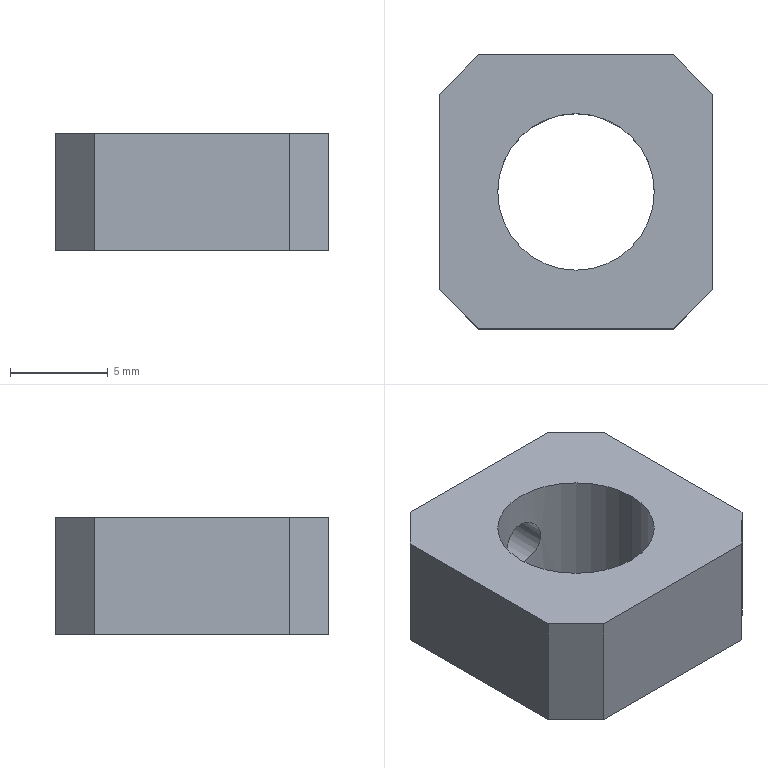Part | SolidWorks | features 3DProfileFeature 1, Chamfer 1, Extrusion 1, HoleWzd 1 | 1 solid | 14 faces | box 14 x 14 x 6 mm | volume 811.438 mm3 | plane 10 | cylinder 4 | commonest cylinder face diameters 2.5 x2 8 x2
STEP:
#1=CARTESIAN_POINT('',(0.,4.,1.25));
#2=VERTEX_POINT('',#1);
#3=CARTESIAN_POINT('',(0.,4.,-1.25));
#4=VERTEX_POINT('',#3);
#5=CARTESIAN_POINT('',(0.,4.,1.25));
#6=CARTESIAN_POINT('',(-0.1663,4.,1.25));
#7=CARTESIAN_POINT('',(-0.3294,3.989,1.217));
#8=CARTESIAN_POINT('',(-0.6318,3.953,1.091));
#9=CARTESIAN_POINT('',(-0.7697,3.927,0.9981));
#10=CARTESIAN_POINT('',(-0.9987,3.875,0.7689));
#11=CARTESIAN_POINT('',(-1.092,3.849,0.6304));
#12=CARTESIAN_POINT('',(-1.217,3.811,0.33));
#13=CARTESIAN_POINT('',(-1.25,3.8,0.1648));
#14=CARTESIAN_POINT('',(-1.25,3.8,-0.08153));
#15=CARTESIAN_POINT('',(-1.242,3.802,-0.165));
#16=CARTESIAN_POINT('',(-1.21,3.813,-0.3257));
#17=CARTESIAN_POINT('',(-1.186,3.82,-0.4039));
#18=CARTESIAN_POINT('',(-1.091,3.849,-0.6319));
#19=CARTESIAN_POINT('',(-0.9989,3.875,-0.769));
#20=CARTESIAN_POINT('',(-0.8259,3.914,-0.9418));
#21=CARTESIAN_POINT('',(-0.7634,3.927,-0.9932));
#22=CARTESIAN_POINT('',(-0.6283,3.951,-1.084));
#23=CARTESIAN_POINT('',(-0.5551,3.962,-1.123));
#24=CARTESIAN_POINT('',(-0.3291,3.989,-1.217));
#25=CARTESIAN_POINT('',(-0.1639,4.,-1.25));
#26=CARTESIAN_POINT('',(0.,4.,-1.25));
#27=B_SPLINE_CURVE_WITH_KNOTS('',3,(#5,#6,#7,#8,#9,#10,#11,#12,#13,#14,#15,#16,#17,#18,#19,#20,#21,#22,#23,#24,#25,#26),.UNSPECIFIED.,.F.,.F.,(4,2,2,2,2,2,2,2,2,2,4),(0.,0.0004916,0.0009832,0.001475,0.001966,0.002212,0.002458,0.00295,0.003195,0.003441,0.003933),.UNSPECIFIED.);
#28=EDGE_CURVE('',#2,#4,#27,.T.);
#29=ORIENTED_EDGE('',*,*,#28,.T.);
#30=CARTESIAN_POINT('',(0.,7.,-1.25));
#31=VERTEX_POINT('',#30);
#32=CARTESIAN_POINT('',(0.,7.,-1.25));
#33=DIRECTION('',(0.,1.,0.));
#34=VECTOR('',#33,1000.);
#35=LINE('',#32,#34);
#36=EDGE_CURVE('',#4,#31,#35,.T.);
#37=ORIENTED_EDGE('',*,*,#36,.T.);
#38=CARTESIAN_POINT('',(0.,7.,1.25));
#39=VERTEX_POINT('',#38);
#40=CARTESIAN_POINT('',(0.,7.,0.));
#41=DIRECTION('',(0.,1.,0.));
#42=DIRECTION('',(0.,0.,1.));
#43=AXIS2_PLACEMENT_3D('',#40,#41,#42);
#44=CIRCLE('',#43,1.25);
#45=EDGE_CURVE('',#31,#39,#44,.T.);
#46=ORIENTED_EDGE('',*,*,#45,.T.);
#47=CARTESIAN_POINT('',(0.,7.,1.25));
#48=DIRECTION('',(0.,1.,0.));
#49=VECTOR('',#48,1000.);
#50=LINE('',#47,#49);
#51=EDGE_CURVE('',#2,#39,#50,.T.);
#52=ORIENTED_EDGE('',*,*,#51,.F.);
#53=EDGE_LOOP('',(#29,#37,#46,#52));
#54=FACE_OUTER_BOUND('',#53,.T.);
#55=CARTESIAN_POINT('',(0.,7.,0.));
#56=DIRECTION('',(0.,1.,0.));
#57=DIRECTION('',(0.,0.,1.));
#58=AXIS2_PLACEMENT_3D('',#55,#56,#57);
#59=CYLINDRICAL_SURFACE('',#58,1.25);
#60=ADVANCED_FACE('',(#54),#59,.F.);
#61=CARTESIAN_POINT('',(-4.,0.,3.));
#62=VERTEX_POINT('',#61);
#63=CARTESIAN_POINT('',(4.,0.,3.));
#64=VERTEX_POINT('',#63);
#65=CARTESIAN_POINT('',(0.,0.,3.));
#66=DIRECTION('',(0.,0.,1.));
#67=DIRECTION('',(1.,0.,0.));
#68=AXIS2_PLACEMENT_3D('',#65,#66,#67);
#69=CIRCLE('',#68,4.);
#70=EDGE_CURVE('',#62,#64,#69,.T.);
#71=ORIENTED_EDGE('',*,*,#70,.T.);
#72=CARTESIAN_POINT('',(4.,0.,-3.));
#73=VERTEX_POINT('',#72);
#74=CARTESIAN_POINT('',(4.,0.,3.));
#75=DIRECTION('',(0.,0.,-1.));
#76=VECTOR('',#75,1000.);
#77=LINE('',#74,#76);
#78=EDGE_CURVE('',#64,#73,#77,.T.);
#79=ORIENTED_EDGE('',*,*,#78,.T.);
#80=CARTESIAN_POINT('',(-4.,0.,-3.));
#81=VERTEX_POINT('',#80);
#82=CARTESIAN_POINT('',(0.,0.,-3.));
#83=DIRECTION('',(0.,0.,1.));
#84=DIRECTION('',(1.,0.,0.));
#85=AXIS2_PLACEMENT_3D('',#82,#83,#84);
#86=CIRCLE('',#85,4.);
#87=EDGE_CURVE('',#81,#73,#86,.T.);
#88=ORIENTED_EDGE('',*,*,#87,.F.);
#89=CARTESIAN_POINT('',(-4.,0.,3.));
#90=DIRECTION('',(0.,0.,-1.));
#91=VECTOR('',#90,1000.);
#92=LINE('',#89,#91);
#93=EDGE_CURVE('',#62,#81,#92,.T.);
#94=ORIENTED_EDGE('',*,*,#93,.F.);
#95=EDGE_LOOP('',(#71,#79,#88,#94));
#96=FACE_OUTER_BOUND('',#95,.T.);
#97=CARTESIAN_POINT('',(0.,0.,3.));
#98=DIRECTION('',(0.,0.,-1.));
#99=DIRECTION('',(-1.,0.,0.));
#100=AXIS2_PLACEMENT_3D('',#97,#98,#99);
#101=CYLINDRICAL_SURFACE('',#100,4.);
#102=ADVANCED_FACE('',(#96),#101,.F.);
#103=CARTESIAN_POINT('',(-7.,5.,3.));
#104=VERTEX_POINT('',#103);
#105=CARTESIAN_POINT('',(-7.,-5.,3.));
#106=VERTEX_POINT('',#105);
#107=CARTESIAN_POINT('',(-7.,-7.,3.));
#108=DIRECTION('',(0.,-1.,0.));
#109=VECTOR('',#108,1000.);
#110=LINE('',#107,#109);
#111=EDGE_CURVE('',#104,#106,#110,.T.);
#112=ORIENTED_EDGE('',*,*,#111,.T.);
#113=CARTESIAN_POINT('',(-5.,-7.,3.));
#114=VERTEX_POINT('',#113);
#115=CARTESIAN_POINT('',(-5.,-7.,3.));
#116=DIRECTION('',(0.7071,-0.7071,0.));
#117=VECTOR('',#116,1000.);
#118=LINE('',#115,#117);
#119=EDGE_CURVE('',#106,#114,#118,.T.);
#120=ORIENTED_EDGE('',*,*,#119,.T.);
#121=CARTESIAN_POINT('',(5.,-7.,3.));
#122=VERTEX_POINT('',#121);
#123=CARTESIAN_POINT('',(-7.,-7.,3.));
#124=DIRECTION('',(1.,0.,0.));
#125=VECTOR('',#124,1000.);
#126=LINE('',#123,#125);
#127=EDGE_CURVE('',#114,#122,#126,.T.);
#128=ORIENTED_EDGE('',*,*,#127,.T.);
#129=CARTESIAN_POINT('',(7.,-5.,3.));
#130=VERTEX_POINT('',#129);
#131=CARTESIAN_POINT('',(7.,-5.,3.));
#132=DIRECTION('',(0.7071,0.7071,0.));
#133=VECTOR('',#132,1000.);
#134=LINE('',#131,#133);
#135=EDGE_CURVE('',#122,#130,#134,.T.);
#136=ORIENTED_EDGE('',*,*,#135,.T.);
#137=CARTESIAN_POINT('',(7.,5.,3.));
#138=VERTEX_POINT('',#137);
#139=CARTESIAN_POINT('',(7.,-7.,3.));
#140=DIRECTION('',(0.,1.,0.));
#141=VECTOR('',#140,1000.);
#142=LINE('',#139,#141);
#143=EDGE_CURVE('',#130,#138,#142,.T.);
#144=ORIENTED_EDGE('',*,*,#143,.T.);
#145=CARTESIAN_POINT('',(5.,7.,3.));
#146=VERTEX_POINT('',#145);
#147=CARTESIAN_POINT('',(5.,7.,3.));
#148=DIRECTION('',(-0.7071,0.7071,0.));
#149=VECTOR('',#148,1000.);
#150=LINE('',#147,#149);
#151=EDGE_CURVE('',#138,#146,#150,.T.);
#152=ORIENTED_EDGE('',*,*,#151,.T.);
#153=CARTESIAN_POINT('',(-5.,7.,3.));
#154=VERTEX_POINT('',#153);
#155=CARTESIAN_POINT('',(-7.,7.,3.));
#156=DIRECTION('',(-1.,0.,0.));
#157=VECTOR('',#156,1000.);
#158=LINE('',#155,#157);
#159=EDGE_CURVE('',#146,#154,#158,.T.);
#160=ORIENTED_EDGE('',*,*,#159,.T.);
#161=CARTESIAN_POINT('',(-7.,5.,3.));
#162=DIRECTION('',(-0.7071,-0.7071,0.));
#163=VECTOR('',#162,1000.);
#164=LINE('',#161,#163);
#165=EDGE_CURVE('',#154,#104,#164,.T.);
#166=ORIENTED_EDGE('',*,*,#165,.T.);
#167=EDGE_LOOP('',(#112,#120,#128,#136,#144,#152,#160,#166));
#168=FACE_OUTER_BOUND('',#167,.T.);
#169=ORIENTED_EDGE('',*,*,#70,.F.);
#170=CARTESIAN_POINT('',(0.,0.,3.));
#171=DIRECTION('',(0.,0.,1.));
#172=DIRECTION('',(1.,0.,0.));
#173=AXIS2_PLACEMENT_3D('',#170,#171,#172);
#174=CIRCLE('',#173,4.);
#175=EDGE_CURVE('',#64,#62,#174,.T.);
#176=ORIENTED_EDGE('',*,*,#175,.F.);
#177=EDGE_LOOP('',(#169,#176));
#178=FACE_BOUND('',#177,.T.);
#179=CARTESIAN_POINT('',(0.,0.,3.));
#180=DIRECTION('',(0.,0.,-1.));
#181=DIRECTION('',(-1.,0.,0.));
#182=AXIS2_PLACEMENT_3D('',#179,#180,#181);
#183=PLANE('',#182);
#184=ADVANCED_FACE('',(#168,#178),#183,.F.);
#185=CARTESIAN_POINT('',(-5.,-7.,-3.));
#186=VERTEX_POINT('',#185);
#187=CARTESIAN_POINT('',(5.,-7.,-3.));
#188=VERTEX_POINT('',#187);
#189=CARTESIAN_POINT('',(-7.,-7.,-3.));
#190=DIRECTION('',(1.,0.,0.));
#191=VECTOR('',#190,1000.);
#192=LINE('',#189,#191);
#193=EDGE_CURVE('',#186,#188,#192,.T.);
#194=ORIENTED_EDGE('',*,*,#193,.F.);
#195=CARTESIAN_POINT('',(-7.,-5.,-3.));
#196=VERTEX_POINT('',#195);
#197=CARTESIAN_POINT('',(-6.,-6.,-3.));
#198=DIRECTION('',(-0.7071,0.7071,0.));
#199=VECTOR('',#198,1000.);
#200=LINE('',#197,#199);
#201=EDGE_CURVE('',#186,#196,#200,.T.);
#202=ORIENTED_EDGE('',*,*,#201,.T.);
#203=CARTESIAN_POINT('',(-7.,5.,-3.));
#204=VERTEX_POINT('',#203);
#205=CARTESIAN_POINT('',(-7.,-7.,-3.));
#206=DIRECTION('',(0.,-1.,0.));
#207=VECTOR('',#206,1000.);
#208=LINE('',#205,#207);
#209=EDGE_CURVE('',#204,#196,#208,.T.);
#210=ORIENTED_EDGE('',*,*,#209,.F.);
#211=CARTESIAN_POINT('',(-5.,7.,-3.));
#212=VERTEX_POINT('',#211);
#213=CARTESIAN_POINT('',(-6.,6.,-3.));
#214=DIRECTION('',(0.7071,0.7071,0.));
#215=VECTOR('',#214,1000.);
#216=LINE('',#213,#215);
#217=EDGE_CURVE('',#204,#212,#216,.T.);
#218=ORIENTED_EDGE('',*,*,#217,.T.);
#219=CARTESIAN_POINT('',(5.,7.,-3.));
#220=VERTEX_POINT('',#219);
#221=CARTESIAN_POINT('',(-7.,7.,-3.));
#222=DIRECTION('',(-1.,0.,0.));
#223=VECTOR('',#222,1000.);
#224=LINE('',#221,#223);
#225=EDGE_CURVE('',#220,#212,#224,.T.);
#226=ORIENTED_EDGE('',*,*,#225,.F.);
#227=CARTESIAN_POINT('',(7.,5.,-3.));
#228=VERTEX_POINT('',#227);
#229=CARTESIAN_POINT('',(6.,6.,-3.));
#230=DIRECTION('',(0.7071,-0.7071,0.));
#231=VECTOR('',#230,1000.);
#232=LINE('',#229,#231);
#233=EDGE_CURVE('',#220,#228,#232,.T.);
#234=ORIENTED_EDGE('',*,*,#233,.T.);
#235=CARTESIAN_POINT('',(7.,-5.,-3.));
#236=VERTEX_POINT('',#235);
#237=CARTESIAN_POINT('',(7.,-7.,-3.));
#238=DIRECTION('',(0.,1.,0.));
#239=VECTOR('',#238,1000.);
#240=LINE('',#237,#239);
#241=EDGE_CURVE('',#236,#228,#240,.T.);
#242=ORIENTED_EDGE('',*,*,#241,.F.);
#243=CARTESIAN_POINT('',(6.,-6.,-3.));
#244=DIRECTION('',(-0.7071,-0.7071,0.));
#245=VECTOR('',#244,1000.);
#246=LINE('',#243,#245);
#247=EDGE_CURVE('',#236,#188,#246,.T.);
#248=ORIENTED_EDGE('',*,*,#247,.T.);
#249=EDGE_LOOP('',(#194,#202,#210,#218,#226,#234,#242,#248));
#250=FACE_OUTER_BOUND('',#249,.T.);
#251=ORIENTED_EDGE('',*,*,#87,.T.);
#252=CARTESIAN_POINT('',(0.,0.,-3.));
#253=DIRECTION('',(0.,0.,1.));
#254=DIRECTION('',(1.,0.,0.));
#255=AXIS2_PLACEMENT_3D('',#252,#253,#254);
#256=CIRCLE('',#255,4.);
#257=EDGE_CURVE('',#73,#81,#256,.T.);
#258=ORIENTED_EDGE('',*,*,#257,.T.);
#259=EDGE_LOOP('',(#251,#258));
#260=FACE_BOUND('',#259,.T.);
#261=CARTESIAN_POINT('',(0.,0.,-3.));
#262=DIRECTION('',(0.,0.,-1.));
#263=DIRECTION('',(-1.,0.,0.));
#264=AXIS2_PLACEMENT_3D('',#261,#262,#263);
#265=PLANE('',#264);
#266=ADVANCED_FACE('',(#250,#260),#265,.T.);
#267=ORIENTED_EDGE('',*,*,#143,.F.);
#268=CARTESIAN_POINT('',(7.,-5.,3.));
#269=DIRECTION('',(0.,0.,-1.));
#270=VECTOR('',#269,1000.);
#271=LINE('',#268,#270);
#272=EDGE_CURVE('',#130,#236,#271,.T.);
#273=ORIENTED_EDGE('',*,*,#272,.T.);
#274=ORIENTED_EDGE('',*,*,#241,.T.);
#275=CARTESIAN_POINT('',(7.,5.,3.));
#276=DIRECTION('',(0.,0.,1.));
#277=VECTOR('',#276,1000.);
#278=LINE('',#275,#277);
#279=EDGE_CURVE('',#228,#138,#278,.T.);
#280=ORIENTED_EDGE('',*,*,#279,.T.);
#281=EDGE_LOOP('',(#267,#273,#274,#280));
#282=FACE_OUTER_BOUND('',#281,.T.);
#283=CARTESIAN_POINT('',(7.,-7.,3.));
#284=DIRECTION('',(-1.,0.,0.));
#285=DIRECTION('',(0.,0.,1.));
#286=AXIS2_PLACEMENT_3D('',#283,#284,#285);
#287=PLANE('',#286);
#288=ADVANCED_FACE('',(#282),#287,.F.);
#289=CARTESIAN_POINT('',(0.,7.,0.));
#290=DIRECTION('',(0.,1.,0.));
#291=DIRECTION('',(0.,0.,1.));
#292=AXIS2_PLACEMENT_3D('',#289,#290,#291);
#293=CIRCLE('',#292,1.25);
#294=EDGE_CURVE('',#39,#31,#293,.T.);
#295=ORIENTED_EDGE('',*,*,#294,.F.);
#296=ORIENTED_EDGE('',*,*,#45,.F.);
#297=EDGE_LOOP('',(#295,#296));
#298=FACE_BOUND('',#297,.T.);
#299=ORIENTED_EDGE('',*,*,#159,.F.);
#300=CARTESIAN_POINT('',(5.,7.,3.));
#301=DIRECTION('',(0.,0.,-1.));
#302=VECTOR('',#301,1000.);
#303=LINE('',#300,#302);
#304=EDGE_CURVE('',#146,#220,#303,.T.);
#305=ORIENTED_EDGE('',*,*,#304,.T.);
#306=ORIENTED_EDGE('',*,*,#225,.T.);
#307=CARTESIAN_POINT('',(-5.,7.,3.));
#308=DIRECTION('',(0.,0.,1.));
#309=VECTOR('',#308,1000.);
#310=LINE('',#307,#309);
#311=EDGE_CURVE('',#212,#154,#310,.T.);
#312=ORIENTED_EDGE('',*,*,#311,.T.);
#313=EDGE_LOOP('',(#299,#305,#306,#312));
#314=FACE_OUTER_BOUND('',#313,.T.);
#315=CARTESIAN_POINT('',(-7.,7.,3.));
#316=DIRECTION('',(0.,-1.,0.));
#317=DIRECTION('',(0.,0.,-1.));
#318=AXIS2_PLACEMENT_3D('',#315,#316,#317);
#319=PLANE('',#318);
#320=ADVANCED_FACE('',(#298,#314),#319,.F.);
#321=ORIENTED_EDGE('',*,*,#209,.T.);
#322=CARTESIAN_POINT('',(-7.,-5.,3.));
#323=DIRECTION('',(0.,0.,1.));
#324=VECTOR('',#323,1000.);
#325=LINE('',#322,#324);
#326=EDGE_CURVE('',#196,#106,#325,.T.);
#327=ORIENTED_EDGE('',*,*,#326,.T.);
#328=ORIENTED_EDGE('',*,*,#111,.F.);
#329=CARTESIAN_POINT('',(-7.,5.,3.));
#330=DIRECTION('',(0.,0.,-1.));
#331=VECTOR('',#330,1000.);
#332=LINE('',#329,#331);
#333=EDGE_CURVE('',#104,#204,#332,.T.);
#334=ORIENTED_EDGE('',*,*,#333,.T.);
#335=EDGE_LOOP('',(#321,#327,#328,#334));
#336=FACE_OUTER_BOUND('',#335,.T.);
#337=CARTESIAN_POINT('',(-7.,-7.,3.));
#338=DIRECTION('',(1.,0.,0.));
#339=DIRECTION('',(0.,0.,-1.));
#340=AXIS2_PLACEMENT_3D('',#337,#338,#339);
#341=PLANE('',#340);
#342=ADVANCED_FACE('',(#336),#341,.F.);
#343=ORIENTED_EDGE('',*,*,#127,.F.);
#344=CARTESIAN_POINT('',(-5.,-7.,3.));
#345=DIRECTION('',(0.,0.,-1.));
#346=VECTOR('',#345,1000.);
#347=LINE('',#344,#346);
#348=EDGE_CURVE('',#114,#186,#347,.T.);
#349=ORIENTED_EDGE('',*,*,#348,.T.);
#350=ORIENTED_EDGE('',*,*,#193,.T.);
#351=CARTESIAN_POINT('',(5.,-7.,3.));
#352=DIRECTION('',(0.,0.,1.));
#353=VECTOR('',#352,1000.);
#354=LINE('',#351,#353);
#355=EDGE_CURVE('',#188,#122,#354,.T.);
#356=ORIENTED_EDGE('',*,*,#355,.T.);
#357=EDGE_LOOP('',(#343,#349,#350,#356));
#358=FACE_OUTER_BOUND('',#357,.T.);
#359=CARTESIAN_POINT('',(-7.,-7.,3.));
#360=DIRECTION('',(0.,1.,0.));
#361=DIRECTION('',(0.,0.,1.));
#362=AXIS2_PLACEMENT_3D('',#359,#360,#361);
#363=PLANE('',#362);
#364=ADVANCED_FACE('',(#358),#363,.F.);
#365=ORIENTED_EDGE('',*,*,#78,.F.);
#366=ORIENTED_EDGE('',*,*,#175,.T.);
#367=ORIENTED_EDGE('',*,*,#93,.T.);
#368=ORIENTED_EDGE('',*,*,#257,.F.);
#369=EDGE_LOOP('',(#365,#366,#367,#368));
#370=FACE_OUTER_BOUND('',#369,.T.);
#371=ORIENTED_EDGE('',*,*,#28,.F.);
#372=CARTESIAN_POINT('',(0.,4.,-1.25));
#373=CARTESIAN_POINT('',(0.1638,4.,-1.25));
#374=CARTESIAN_POINT('',(0.3292,3.989,-1.217));
#375=CARTESIAN_POINT('',(0.6307,3.953,-1.092));
#376=CARTESIAN_POINT('',(0.7685,3.927,-0.9993));
#377=CARTESIAN_POINT('',(0.9992,3.875,-0.7685));
#378=CARTESIAN_POINT('',(1.091,3.849,-0.6322));
#379=CARTESIAN_POINT('',(1.186,3.82,-0.404));
#380=CARTESIAN_POINT('',(1.21,3.813,-0.3259));
#381=CARTESIAN_POINT('',(1.242,3.802,-0.1656));
#382=CARTESIAN_POINT('',(1.25,3.8,-0.08239));
#383=CARTESIAN_POINT('',(1.25,3.8,0.1647));
#384=CARTESIAN_POINT('',(1.217,3.811,0.3295));
#385=CARTESIAN_POINT('',(1.092,3.849,0.6305));
#386=CARTESIAN_POINT('',(0.9987,3.875,0.769));
#387=CARTESIAN_POINT('',(0.7696,3.927,0.9982));
#388=CARTESIAN_POINT('',(0.6317,3.953,1.091));
#389=CARTESIAN_POINT('',(0.3299,3.989,1.217));
#390=CARTESIAN_POINT('',(0.1663,4.,1.25));
#391=CARTESIAN_POINT('',(0.,4.,1.25));
#392=B_SPLINE_CURVE_WITH_KNOTS('',3,(#372,#373,#374,#375,#376,#377,#378,#379,#380,#381,#382,#383,#384,#385,#386,#387,#388,#389,#390,#391),.UNSPECIFIED.,.F.,.F.,(4,2,2,2,2,2,2,2,2,4),(0.003933,0.004424,0.004916,0.005407,0.005653,0.005899,0.00639,0.006882,0.007373,0.007865),.UNSPECIFIED.);
#393=EDGE_CURVE('',#4,#2,#392,.T.);
#394=ORIENTED_EDGE('',*,*,#393,.F.);
#395=EDGE_LOOP('',(#371,#394));
#396=FACE_BOUND('',#395,.T.);
#397=CARTESIAN_POINT('',(0.,0.,3.));
#398=DIRECTION('',(0.,0.,-1.));
#399=DIRECTION('',(-1.,0.,0.));
#400=AXIS2_PLACEMENT_3D('',#397,#398,#399);
#401=CYLINDRICAL_SURFACE('',#400,4.);
#402=ADVANCED_FACE('',(#370,#396),#401,.F.);
#403=ORIENTED_EDGE('',*,*,#36,.F.);
#404=ORIENTED_EDGE('',*,*,#393,.T.);
#405=ORIENTED_EDGE('',*,*,#51,.T.);
#406=ORIENTED_EDGE('',*,*,#294,.T.);
#407=EDGE_LOOP('',(#403,#404,#405,#406));
#408=FACE_OUTER_BOUND('',#407,.T.);
#409=CARTESIAN_POINT('',(0.,7.,0.));
#410=DIRECTION('',(0.,1.,0.));
#411=DIRECTION('',(0.,0.,1.));
#412=AXIS2_PLACEMENT_3D('',#409,#410,#411);
#413=CYLINDRICAL_SURFACE('',#412,1.25);
#414=ADVANCED_FACE('',(#408),#413,.F.);
#415=ORIENTED_EDGE('',*,*,#119,.F.);
#416=ORIENTED_EDGE('',*,*,#326,.F.);
#417=ORIENTED_EDGE('',*,*,#201,.F.);
#418=ORIENTED_EDGE('',*,*,#348,.F.);
#419=EDGE_LOOP('',(#415,#416,#417,#418));
#420=FACE_OUTER_BOUND('',#419,.T.);
#421=CARTESIAN_POINT('',(-5.,-7.,3.));
#422=DIRECTION('',(0.7071,0.7071,0.));
#423=DIRECTION('',(0.,0.,-1.));
#424=AXIS2_PLACEMENT_3D('',#421,#422,#423);
#425=PLANE('',#424);
#426=ADVANCED_FACE('',(#420),#425,.F.);
#427=ORIENTED_EDGE('',*,*,#135,.F.);
#428=ORIENTED_EDGE('',*,*,#355,.F.);
#429=ORIENTED_EDGE('',*,*,#247,.F.);
#430=ORIENTED_EDGE('',*,*,#272,.F.);
#431=EDGE_LOOP('',(#427,#428,#429,#430));
#432=FACE_OUTER_BOUND('',#431,.T.);
#433=CARTESIAN_POINT('',(7.,-5.,3.));
#434=DIRECTION('',(-0.7071,0.7071,0.));
#435=DIRECTION('',(0.,0.,-1.));
#436=AXIS2_PLACEMENT_3D('',#433,#434,#435);
#437=PLANE('',#436);
#438=ADVANCED_FACE('',(#432),#437,.F.);
#439=ORIENTED_EDGE('',*,*,#151,.F.);
#440=ORIENTED_EDGE('',*,*,#279,.F.);
#441=ORIENTED_EDGE('',*,*,#233,.F.);
#442=ORIENTED_EDGE('',*,*,#304,.F.);
#443=EDGE_LOOP('',(#439,#440,#441,#442));
#444=FACE_OUTER_BOUND('',#443,.T.);
#445=CARTESIAN_POINT('',(5.,7.,3.));
#446=DIRECTION('',(-0.7071,-0.7071,0.));
#447=DIRECTION('',(0.,0.,-1.));
#448=AXIS2_PLACEMENT_3D('',#445,#446,#447);
#449=PLANE('',#448);
#450=ADVANCED_FACE('',(#444),#449,.F.);
#451=ORIENTED_EDGE('',*,*,#165,.F.);
#452=ORIENTED_EDGE('',*,*,#311,.F.);
#453=ORIENTED_EDGE('',*,*,#217,.F.);
#454=ORIENTED_EDGE('',*,*,#333,.F.);
#455=EDGE_LOOP('',(#451,#452,#453,#454));
#456=FACE_OUTER_BOUND('',#455,.T.);
#457=CARTESIAN_POINT('',(-7.,5.,3.));
#458=DIRECTION('',(0.7071,-0.7071,0.));
#459=DIRECTION('',(0.,0.,-1.));
#460=AXIS2_PLACEMENT_3D('',#457,#458,#459);
#461=PLANE('',#460);
#462=ADVANCED_FACE('',(#456),#461,.F.);
#463=CLOSED_SHELL('',(#60,#102,#184,#266,#288,#320,#342,#364,#402,#414,#426,#438,#450,#462));
#464=MANIFOLD_SOLID_BREP('',#463);
#465=CARTESIAN_POINT('',(0.,0.,0.));
#466=DIRECTION('',(0.,0.,1.));
#467=DIRECTION('',(1.,0.,0.));
#468=AXIS2_PLACEMENT_3D('',#465,#466,#467);
#469=(LENGTH_UNIT()NAMED_UNIT(*)SI_UNIT(.MILLI.,.METRE.));
#470=UNCERTAINTY_MEASURE_WITH_UNIT(LENGTH_MEASURE(0.00001),#469,'','');
#471=(NAMED_UNIT(*)PLANE_ANGLE_UNIT()SI_UNIT($,.RADIAN.));
#472=(NAMED_UNIT(*)SI_UNIT($,.STERADIAN.)SOLID_ANGLE_UNIT());
#473=(GEOMETRIC_REPRESENTATION_CONTEXT(3)GLOBAL_UNCERTAINTY_ASSIGNED_CONTEXT((#470))GLOBAL_UNIT_ASSIGNED_CONTEXT((#469,#471,#472))REPRESENTATION_CONTEXT('',''));
#474=ADVANCED_BREP_SHAPE_REPRESENTATION('',(#464,#468),#473);